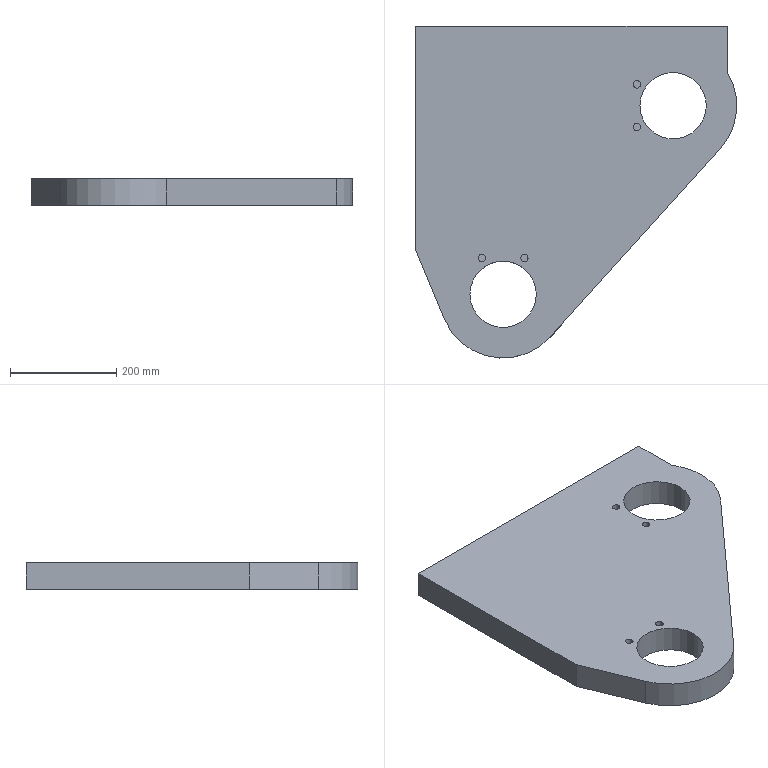Part | SolidWorks | features Cut 1, SplitBody 1 | 1 solid | 25 faces | box 605 x 625 x 50 mm | volume 12901911 mm3 | cylinder 14 | plane 11 | commonest cylinder face diameters 14 x8 125 x4 240 x2
STEP:
#1=CARTESIAN_POINT('',(3069.,481.749,-775.));
#2=VERTEX_POINT('',#1);
#3=CARTESIAN_POINT('',(3083.,481.749,-775.));
#4=VERTEX_POINT('',#3);
#5=CARTESIAN_POINT('',(3076.,481.749,-775.));
#6=DIRECTION('',(0.,0.,1.));
#7=DIRECTION('',(-1.,0.,0.));
#8=AXIS2_PLACEMENT_3D('',#5,#6,#7);
#9=CIRCLE('',#8,7.);
#10=EDGE_CURVE('',#2,#4,#9,.T.);
#11=ORIENTED_EDGE('',*,*,#10,.F.);
#12=CARTESIAN_POINT('',(3069.,481.749,-755.));
#13=VERTEX_POINT('',#12);
#14=CARTESIAN_POINT('',(3069.,481.749,-775.));
#15=DIRECTION('',(0.,0.,1.));
#16=VECTOR('',#15,1000.);
#17=LINE('',#14,#16);
#18=EDGE_CURVE('',#2,#13,#17,.T.);
#19=ORIENTED_EDGE('',*,*,#18,.T.);
#20=CARTESIAN_POINT('',(3083.,481.749,-755.));
#21=VERTEX_POINT('',#20);
#22=CARTESIAN_POINT('',(3076.,481.749,-755.));
#23=DIRECTION('',(0.,0.,1.));
#24=DIRECTION('',(-1.,0.,0.));
#25=AXIS2_PLACEMENT_3D('',#22,#23,#24);
#26=CIRCLE('',#25,7.);
#27=EDGE_CURVE('',#13,#21,#26,.T.);
#28=ORIENTED_EDGE('',*,*,#27,.T.);
#29=CARTESIAN_POINT('',(3083.,481.749,-775.));
#30=DIRECTION('',(0.,0.,1.));
#31=VECTOR('',#30,1000.);
#32=LINE('',#29,#31);
#33=EDGE_CURVE('',#4,#21,#32,.T.);
#34=ORIENTED_EDGE('',*,*,#33,.F.);
#35=EDGE_LOOP('',(#11,#19,#28,#34));
#36=FACE_OUTER_BOUND('',#35,.T.);
#37=CARTESIAN_POINT('',(3076.,481.749,-775.));
#38=DIRECTION('',(0.,0.,1.));
#39=DIRECTION('',(1.,0.,0.));
#40=AXIS2_PLACEMENT_3D('',#37,#38,#39);
#41=CYLINDRICAL_SURFACE('',#40,7.);
#42=ADVANCED_FACE('',(#36),#41,.F.);
#43=CARTESIAN_POINT('',(3149.,481.749,-775.));
#44=VERTEX_POINT('',#43);
#45=CARTESIAN_POINT('',(3163.,481.749,-775.));
#46=VERTEX_POINT('',#45);
#47=CARTESIAN_POINT('',(3156.,481.749,-775.));
#48=DIRECTION('',(0.,0.,1.));
#49=DIRECTION('',(1.,0.,0.));
#50=AXIS2_PLACEMENT_3D('',#47,#48,#49);
#51=CIRCLE('',#50,7.);
#52=EDGE_CURVE('',#44,#46,#51,.T.);
#53=ORIENTED_EDGE('',*,*,#52,.F.);
#54=CARTESIAN_POINT('',(3149.,481.749,-755.));
#55=VERTEX_POINT('',#54);
#56=CARTESIAN_POINT('',(3149.,481.749,-775.));
#57=DIRECTION('',(0.,0.,1.));
#58=VECTOR('',#57,1000.);
#59=LINE('',#56,#58);
#60=EDGE_CURVE('',#44,#55,#59,.T.);
#61=ORIENTED_EDGE('',*,*,#60,.T.);
#62=CARTESIAN_POINT('',(3163.,481.749,-755.));
#63=VERTEX_POINT('',#62);
#64=CARTESIAN_POINT('',(3156.,481.749,-755.));
#65=DIRECTION('',(0.,0.,1.));
#66=DIRECTION('',(1.,0.,0.));
#67=AXIS2_PLACEMENT_3D('',#64,#65,#66);
#68=CIRCLE('',#67,7.);
#69=EDGE_CURVE('',#55,#63,#68,.T.);
#70=ORIENTED_EDGE('',*,*,#69,.T.);
#71=CARTESIAN_POINT('',(3163.,481.749,-775.));
#72=DIRECTION('',(0.,0.,1.));
#73=VECTOR('',#72,1000.);
#74=LINE('',#71,#73);
#75=EDGE_CURVE('',#46,#63,#74,.T.);
#76=ORIENTED_EDGE('',*,*,#75,.F.);
#77=EDGE_LOOP('',(#53,#61,#70,#76));
#78=FACE_OUTER_BOUND('',#77,.T.);
#79=CARTESIAN_POINT('',(3156.,481.749,-775.));
#80=DIRECTION('',(0.,0.,1.));
#81=DIRECTION('',(1.,0.,0.));
#82=AXIS2_PLACEMENT_3D('',#79,#80,#81);
#83=CYLINDRICAL_SURFACE('',#82,7.);
#84=ADVANCED_FACE('',(#78),#83,.F.);
#85=CARTESIAN_POINT('',(3360.692,808.44,-775.));
#86=VERTEX_POINT('',#85);
#87=CARTESIAN_POINT('',(3374.692,808.44,-775.));
#88=VERTEX_POINT('',#87);
#89=CARTESIAN_POINT('',(3367.692,808.44,-775.));
#90=DIRECTION('',(0.,0.,1.));
#91=DIRECTION('',(1.,0.,0.));
#92=AXIS2_PLACEMENT_3D('',#89,#90,#91);
#93=CIRCLE('',#92,7.);
#94=EDGE_CURVE('',#86,#88,#93,.T.);
#95=ORIENTED_EDGE('',*,*,#94,.F.);
#96=CARTESIAN_POINT('',(3360.692,808.44,-755.));
#97=VERTEX_POINT('',#96);
#98=CARTESIAN_POINT('',(3360.692,808.44,-775.));
#99=DIRECTION('',(0.,0.,1.));
#100=VECTOR('',#99,1000.);
#101=LINE('',#98,#100);
#102=EDGE_CURVE('',#86,#97,#101,.T.);
#103=ORIENTED_EDGE('',*,*,#102,.T.);
#104=CARTESIAN_POINT('',(3374.692,808.44,-755.));
#105=VERTEX_POINT('',#104);
#106=CARTESIAN_POINT('',(3367.692,808.44,-755.));
#107=DIRECTION('',(0.,0.,1.));
#108=DIRECTION('',(1.,0.,0.));
#109=AXIS2_PLACEMENT_3D('',#106,#107,#108);
#110=CIRCLE('',#109,7.);
#111=EDGE_CURVE('',#97,#105,#110,.T.);
#112=ORIENTED_EDGE('',*,*,#111,.T.);
#113=CARTESIAN_POINT('',(3374.692,808.44,-775.));
#114=DIRECTION('',(0.,0.,1.));
#115=VECTOR('',#114,1000.);
#116=LINE('',#113,#115);
#117=EDGE_CURVE('',#88,#105,#116,.T.);
#118=ORIENTED_EDGE('',*,*,#117,.F.);
#119=EDGE_LOOP('',(#95,#103,#112,#118));
#120=FACE_OUTER_BOUND('',#119,.T.);
#121=CARTESIAN_POINT('',(3367.692,808.44,-775.));
#122=DIRECTION('',(0.,0.,1.));
#123=DIRECTION('',(1.,0.,0.));
#124=AXIS2_PLACEMENT_3D('',#121,#122,#123);
#125=CYLINDRICAL_SURFACE('',#124,7.);
#126=ADVANCED_FACE('',(#120),#125,.F.);
#127=CARTESIAN_POINT('',(3360.692,728.44,-775.));
#128=VERTEX_POINT('',#127);
#129=CARTESIAN_POINT('',(3374.692,728.44,-775.));
#130=VERTEX_POINT('',#129);
#131=CARTESIAN_POINT('',(3367.692,728.44,-775.));
#132=DIRECTION('',(0.,0.,1.));
#133=DIRECTION('',(1.,0.,0.));
#134=AXIS2_PLACEMENT_3D('',#131,#132,#133);
#135=CIRCLE('',#134,7.);
#136=EDGE_CURVE('',#128,#130,#135,.T.);
#137=ORIENTED_EDGE('',*,*,#136,.F.);
#138=CARTESIAN_POINT('',(3360.692,728.44,-755.));
#139=VERTEX_POINT('',#138);
#140=CARTESIAN_POINT('',(3360.692,728.44,-775.));
#141=DIRECTION('',(0.,0.,1.));
#142=VECTOR('',#141,1000.);
#143=LINE('',#140,#142);
#144=EDGE_CURVE('',#128,#139,#143,.T.);
#145=ORIENTED_EDGE('',*,*,#144,.T.);
#146=CARTESIAN_POINT('',(3374.692,728.44,-755.));
#147=VERTEX_POINT('',#146);
#148=CARTESIAN_POINT('',(3367.692,728.44,-755.));
#149=DIRECTION('',(0.,0.,1.));
#150=DIRECTION('',(1.,0.,0.));
#151=AXIS2_PLACEMENT_3D('',#148,#149,#150);
#152=CIRCLE('',#151,7.);
#153=EDGE_CURVE('',#139,#147,#152,.T.);
#154=ORIENTED_EDGE('',*,*,#153,.T.);
#155=CARTESIAN_POINT('',(3374.692,728.44,-775.));
#156=DIRECTION('',(0.,0.,1.));
#157=VECTOR('',#156,1000.);
#158=LINE('',#155,#157);
#159=EDGE_CURVE('',#130,#147,#158,.T.);
#160=ORIENTED_EDGE('',*,*,#159,.F.);
#161=EDGE_LOOP('',(#137,#145,#154,#160));
#162=FACE_OUTER_BOUND('',#161,.T.);
#163=CARTESIAN_POINT('',(3367.692,728.44,-775.));
#164=DIRECTION('',(0.,0.,1.));
#165=DIRECTION('',(1.,0.,0.));
#166=AXIS2_PLACEMENT_3D('',#163,#164,#165);
#167=CYLINDRICAL_SURFACE('',#166,7.);
#168=ADVANCED_FACE('',(#162),#167,.F.);
#169=CARTESIAN_POINT('',(3178.5,413.44,-755.));
#170=VERTEX_POINT('',#169);
#171=CARTESIAN_POINT('',(3053.5,413.44,-755.));
#172=VERTEX_POINT('',#171);
#173=CARTESIAN_POINT('',(3116.,413.44,-755.));
#174=DIRECTION('',(0.,0.,-1.));
#175=DIRECTION('',(-1.,0.,0.));
#176=AXIS2_PLACEMENT_3D('',#173,#174,#175);
#177=CIRCLE('',#176,62.5);
#178=EDGE_CURVE('',#170,#172,#177,.T.);
#179=ORIENTED_EDGE('',*,*,#178,.F.);
#180=CARTESIAN_POINT('',(3178.5,413.44,-805.));
#181=VERTEX_POINT('',#180);
#182=CARTESIAN_POINT('',(3178.5,413.44,-755.));
#183=DIRECTION('',(0.,0.,-1.));
#184=VECTOR('',#183,1000.);
#185=LINE('',#182,#184);
#186=EDGE_CURVE('',#170,#181,#185,.T.);
#187=ORIENTED_EDGE('',*,*,#186,.T.);
#188=CARTESIAN_POINT('',(3053.5,413.44,-805.));
#189=VERTEX_POINT('',#188);
#190=CARTESIAN_POINT('',(3116.,413.44,-805.));
#191=DIRECTION('',(0.,0.,1.));
#192=DIRECTION('',(-1.,0.,0.));
#193=AXIS2_PLACEMENT_3D('',#190,#191,#192);
#194=CIRCLE('',#193,62.5);
#195=EDGE_CURVE('',#189,#181,#194,.T.);
#196=ORIENTED_EDGE('',*,*,#195,.F.);
#197=CARTESIAN_POINT('',(3053.5,413.44,-755.));
#198=DIRECTION('',(0.,0.,-1.));
#199=VECTOR('',#198,1000.);
#200=LINE('',#197,#199);
#201=EDGE_CURVE('',#172,#189,#200,.T.);
#202=ORIENTED_EDGE('',*,*,#201,.F.);
#203=EDGE_LOOP('',(#179,#187,#196,#202));
#204=FACE_OUTER_BOUND('',#203,.T.);
#205=CARTESIAN_POINT('',(3116.,413.44,-755.));
#206=DIRECTION('',(0.,0.,-1.));
#207=DIRECTION('',(-1.,0.,0.));
#208=AXIS2_PLACEMENT_3D('',#205,#206,#207);
#209=CYLINDRICAL_SURFACE('',#208,62.5);
#210=ADVANCED_FACE('',(#204),#209,.F.);
#211=CARTESIAN_POINT('',(3498.5,768.44,-755.));
#212=VERTEX_POINT('',#211);
#213=CARTESIAN_POINT('',(3373.5,768.44,-755.));
#214=VERTEX_POINT('',#213);
#215=CARTESIAN_POINT('',(3436.,768.44,-755.));
#216=DIRECTION('',(0.,0.,-1.));
#217=DIRECTION('',(-1.,0.,0.));
#218=AXIS2_PLACEMENT_3D('',#215,#216,#217);
#219=CIRCLE('',#218,62.5);
#220=EDGE_CURVE('',#212,#214,#219,.T.);
#221=ORIENTED_EDGE('',*,*,#220,.F.);
#222=CARTESIAN_POINT('',(3498.5,768.44,-805.));
#223=VERTEX_POINT('',#222);
#224=CARTESIAN_POINT('',(3498.5,768.44,-755.));
#225=DIRECTION('',(0.,0.,-1.));
#226=VECTOR('',#225,1000.);
#227=LINE('',#224,#226);
#228=EDGE_CURVE('',#212,#223,#227,.T.);
#229=ORIENTED_EDGE('',*,*,#228,.T.);
#230=CARTESIAN_POINT('',(3373.5,768.44,-805.));
#231=VERTEX_POINT('',#230);
#232=CARTESIAN_POINT('',(3436.,768.44,-805.));
#233=DIRECTION('',(0.,0.,1.));
#234=DIRECTION('',(-1.,0.,0.));
#235=AXIS2_PLACEMENT_3D('',#232,#233,#234);
#236=CIRCLE('',#235,62.5);
#237=EDGE_CURVE('',#231,#223,#236,.T.);
#238=ORIENTED_EDGE('',*,*,#237,.F.);
#239=CARTESIAN_POINT('',(3373.5,768.44,-755.));
#240=DIRECTION('',(0.,0.,-1.));
#241=VECTOR('',#240,1000.);
#242=LINE('',#239,#241);
#243=EDGE_CURVE('',#214,#231,#242,.T.);
#244=ORIENTED_EDGE('',*,*,#243,.F.);
#245=EDGE_LOOP('',(#221,#229,#238,#244));
#246=FACE_OUTER_BOUND('',#245,.T.);
#247=CARTESIAN_POINT('',(3436.,768.44,-755.));
#248=DIRECTION('',(0.,0.,-1.));
#249=DIRECTION('',(-1.,0.,0.));
#250=AXIS2_PLACEMENT_3D('',#247,#248,#249);
#251=CYLINDRICAL_SURFACE('',#250,62.5);
#252=ADVANCED_FACE('',(#246),#251,.F.);
#253=CARTESIAN_POINT('',(3076.,481.749,-755.));
#254=DIRECTION('',(0.,0.,1.));
#255=DIRECTION('',(-1.,0.,0.));
#256=AXIS2_PLACEMENT_3D('',#253,#254,#255);
#257=CIRCLE('',#256,7.);
#258=EDGE_CURVE('',#21,#13,#257,.T.);
#259=ORIENTED_EDGE('',*,*,#258,.F.);
#260=ORIENTED_EDGE('',*,*,#27,.F.);
#261=EDGE_LOOP('',(#259,#260));
#262=FACE_BOUND('',#261,.T.);
#263=CARTESIAN_POINT('',(3156.,481.749,-755.));
#264=DIRECTION('',(0.,0.,1.));
#265=DIRECTION('',(1.,0.,0.));
#266=AXIS2_PLACEMENT_3D('',#263,#264,#265);
#267=CIRCLE('',#266,7.);
#268=EDGE_CURVE('',#63,#55,#267,.T.);
#269=ORIENTED_EDGE('',*,*,#268,.F.);
#270=ORIENTED_EDGE('',*,*,#69,.F.);
#271=EDGE_LOOP('',(#269,#270));
#272=FACE_BOUND('',#271,.T.);
#273=CARTESIAN_POINT('',(3367.692,808.44,-755.));
#274=DIRECTION('',(0.,0.,1.));
#275=DIRECTION('',(1.,0.,0.));
#276=AXIS2_PLACEMENT_3D('',#273,#274,#275);
#277=CIRCLE('',#276,7.);
#278=EDGE_CURVE('',#105,#97,#277,.T.);
#279=ORIENTED_EDGE('',*,*,#278,.F.);
#280=ORIENTED_EDGE('',*,*,#111,.F.);
#281=EDGE_LOOP('',(#279,#280));
#282=FACE_BOUND('',#281,.T.);
#283=CARTESIAN_POINT('',(3367.692,728.44,-755.));
#284=DIRECTION('',(0.,0.,1.));
#285=DIRECTION('',(1.,0.,0.));
#286=AXIS2_PLACEMENT_3D('',#283,#284,#285);
#287=CIRCLE('',#286,7.);
#288=EDGE_CURVE('',#147,#139,#287,.T.);
#289=ORIENTED_EDGE('',*,*,#288,.F.);
#290=ORIENTED_EDGE('',*,*,#153,.F.);
#291=EDGE_LOOP('',(#289,#290));
#292=FACE_BOUND('',#291,.T.);
#293=CARTESIAN_POINT('',(3116.,413.44,-755.));
#294=DIRECTION('',(0.,0.,-1.));
#295=DIRECTION('',(-1.,0.,0.));
#296=AXIS2_PLACEMENT_3D('',#293,#294,#295);
#297=CIRCLE('',#296,62.5);
#298=EDGE_CURVE('',#172,#170,#297,.T.);
#299=ORIENTED_EDGE('',*,*,#298,.T.);
#300=ORIENTED_EDGE('',*,*,#178,.T.);
#301=EDGE_LOOP('',(#299,#300));
#302=FACE_BOUND('',#301,.T.);
#303=CARTESIAN_POINT('',(2951.,918.44,-755.));
#304=VERTEX_POINT('',#303);
#305=CARTESIAN_POINT('',(2951.,498.44,-755.));
#306=VERTEX_POINT('',#305);
#307=CARTESIAN_POINT('',(2951.,413.44,-755.));
#308=DIRECTION('',(0.,-1.,0.));
#309=VECTOR('',#308,1000.);
#310=LINE('',#307,#309);
#311=EDGE_CURVE('',#304,#306,#310,.T.);
#312=ORIENTED_EDGE('',*,*,#311,.T.);
#313=CARTESIAN_POINT('',(3005.106,367.587,-755.));
#314=VERTEX_POINT('',#313);
#315=CARTESIAN_POINT('',(2951.,498.44,-755.));
#316=DIRECTION('',(0.3821,-0.9241,0.));
#317=VECTOR('',#316,1000.);
#318=LINE('',#315,#317);
#319=EDGE_CURVE('',#306,#314,#318,.T.);
#320=ORIENTED_EDGE('',*,*,#319,.T.);
#321=CARTESIAN_POINT('',(3205.133,333.095,-755.));
#322=VERTEX_POINT('',#321);
#323=CARTESIAN_POINT('',(3116.,413.44,-755.));
#324=DIRECTION('',(0.,0.,1.));
#325=DIRECTION('',(-1.,0.,0.));
#326=AXIS2_PLACEMENT_3D('',#323,#324,#325);
#327=CIRCLE('',#326,120.);
#328=EDGE_CURVE('',#314,#322,#327,.T.);
#329=ORIENTED_EDGE('',*,*,#328,.T.);
#330=CARTESIAN_POINT('',(3525.133,688.095,-755.));
#331=VERTEX_POINT('',#330);
#332=CARTESIAN_POINT('',(3205.133,333.095,-755.));
#333=DIRECTION('',(0.6695,0.7428,0.));
#334=VECTOR('',#333,1000.);
#335=LINE('',#332,#334);
#336=EDGE_CURVE('',#322,#331,#335,.T.);
#337=ORIENTED_EDGE('',*,*,#336,.T.);
#338=CARTESIAN_POINT('',(3538.,831.654,-755.));
#339=VERTEX_POINT('',#338);
#340=CARTESIAN_POINT('',(3436.,768.44,-755.));
#341=DIRECTION('',(0.,0.,1.));
#342=DIRECTION('',(-1.,0.,0.));
#343=AXIS2_PLACEMENT_3D('',#340,#341,#342);
#344=CIRCLE('',#343,120.);
#345=EDGE_CURVE('',#331,#339,#344,.T.);
#346=ORIENTED_EDGE('',*,*,#345,.T.);
#347=CARTESIAN_POINT('',(3538.,918.44,-755.));
#348=VERTEX_POINT('',#347);
#349=CARTESIAN_POINT('',(3538.,413.44,-755.));
#350=DIRECTION('',(0.,1.,0.));
#351=VECTOR('',#350,1000.);
#352=LINE('',#349,#351);
#353=EDGE_CURVE('',#339,#348,#352,.T.);
#354=ORIENTED_EDGE('',*,*,#353,.T.);
#355=CARTESIAN_POINT('',(3116.,918.44,-755.));
#356=DIRECTION('',(-1.,0.,0.));
#357=VECTOR('',#356,1000.);
#358=LINE('',#355,#357);
#359=EDGE_CURVE('',#348,#304,#358,.T.);
#360=ORIENTED_EDGE('',*,*,#359,.T.);
#361=EDGE_LOOP('',(#312,#320,#329,#337,#346,#354,#360));
#362=FACE_OUTER_BOUND('',#361,.T.);
#363=CARTESIAN_POINT('',(3436.,768.44,-755.));
#364=DIRECTION('',(0.,0.,-1.));
#365=DIRECTION('',(-1.,0.,0.));
#366=AXIS2_PLACEMENT_3D('',#363,#364,#365);
#367=CIRCLE('',#366,62.5);
#368=EDGE_CURVE('',#214,#212,#367,.T.);
#369=ORIENTED_EDGE('',*,*,#368,.T.);
#370=ORIENTED_EDGE('',*,*,#220,.T.);
#371=EDGE_LOOP('',(#369,#370));
#372=FACE_BOUND('',#371,.T.);
#373=CARTESIAN_POINT('',(3116.,413.44,-755.));
#374=DIRECTION('',(0.,0.,1.));
#375=DIRECTION('',(1.,0.,0.));
#376=AXIS2_PLACEMENT_3D('',#373,#374,#375);
#377=PLANE('',#376);
#378=ADVANCED_FACE('',(#262,#272,#282,#292,#302,#362,#372),#377,.T.);
#379=ORIENTED_EDGE('',*,*,#186,.F.);
#380=ORIENTED_EDGE('',*,*,#298,.F.);
#381=ORIENTED_EDGE('',*,*,#201,.T.);
#382=CARTESIAN_POINT('',(3116.,413.44,-805.));
#383=DIRECTION('',(0.,0.,1.));
#384=DIRECTION('',(-1.,0.,0.));
#385=AXIS2_PLACEMENT_3D('',#382,#383,#384);
#386=CIRCLE('',#385,62.5);
#387=EDGE_CURVE('',#181,#189,#386,.T.);
#388=ORIENTED_EDGE('',*,*,#387,.F.);
#389=EDGE_LOOP('',(#379,#380,#381,#388));
#390=FACE_OUTER_BOUND('',#389,.T.);
#391=CARTESIAN_POINT('',(3116.,413.44,-755.));
#392=DIRECTION('',(0.,0.,-1.));
#393=DIRECTION('',(-1.,0.,0.));
#394=AXIS2_PLACEMENT_3D('',#391,#392,#393);
#395=CYLINDRICAL_SURFACE('',#394,62.5);
#396=ADVANCED_FACE('',(#390),#395,.F.);
#397=CARTESIAN_POINT('',(3005.106,367.587,-805.));
#398=VERTEX_POINT('',#397);
#399=CARTESIAN_POINT('',(3005.106,367.587,-755.));
#400=DIRECTION('',(0.,0.,-1.));
#401=VECTOR('',#400,1000.);
#402=LINE('',#399,#401);
#403=EDGE_CURVE('',#314,#398,#402,.T.);
#404=ORIENTED_EDGE('',*,*,#403,.F.);
#405=ORIENTED_EDGE('',*,*,#319,.F.);
#406=CARTESIAN_POINT('',(2951.,498.44,-805.));
#407=VERTEX_POINT('',#406);
#408=CARTESIAN_POINT('',(2951.,498.44,-755.));
#409=DIRECTION('',(0.,0.,1.));
#410=VECTOR('',#409,1000.);
#411=LINE('',#408,#410);
#412=EDGE_CURVE('',#407,#306,#411,.T.);
#413=ORIENTED_EDGE('',*,*,#412,.F.);
#414=CARTESIAN_POINT('',(2951.,498.44,-805.));
#415=DIRECTION('',(-0.3821,0.9241,0.));
#416=VECTOR('',#415,1000.);
#417=LINE('',#414,#416);
#418=EDGE_CURVE('',#398,#407,#417,.T.);
#419=ORIENTED_EDGE('',*,*,#418,.F.);
#420=EDGE_LOOP('',(#404,#405,#413,#419));
#421=FACE_OUTER_BOUND('',#420,.T.);
#422=CARTESIAN_POINT('',(2951.,498.44,-755.));
#423=DIRECTION('',(0.9241,0.3821,0.));
#424=DIRECTION('',(-0.3821,0.9241,0.));
#425=AXIS2_PLACEMENT_3D('',#422,#423,#424);
#426=PLANE('',#425);
#427=ADVANCED_FACE('',(#421),#426,.F.);
#428=ORIENTED_EDGE('',*,*,#412,.T.);
#429=ORIENTED_EDGE('',*,*,#311,.F.);
#430=CARTESIAN_POINT('',(2951.,918.44,-805.));
#431=VERTEX_POINT('',#430);
#432=CARTESIAN_POINT('',(2951.,918.44,-755.));
#433=DIRECTION('',(0.,0.,1.));
#434=VECTOR('',#433,1000.);
#435=LINE('',#432,#434);
#436=EDGE_CURVE('',#431,#304,#435,.T.);
#437=ORIENTED_EDGE('',*,*,#436,.F.);
#438=CARTESIAN_POINT('',(2951.,498.44,-805.));
#439=DIRECTION('',(0.,1.,0.));
#440=VECTOR('',#439,1000.);
#441=LINE('',#438,#440);
#442=EDGE_CURVE('',#407,#431,#441,.T.);
#443=ORIENTED_EDGE('',*,*,#442,.F.);
#444=EDGE_LOOP('',(#428,#429,#437,#443));
#445=FACE_OUTER_BOUND('',#444,.T.);
#446=CARTESIAN_POINT('',(2951.,498.44,-755.));
#447=DIRECTION('',(1.,0.,0.));
#448=DIRECTION('',(0.,0.,-1.));
#449=AXIS2_PLACEMENT_3D('',#446,#447,#448);
#450=PLANE('',#449);
#451=ADVANCED_FACE('',(#445),#450,.F.);
#452=ORIENTED_EDGE('',*,*,#436,.T.);
#453=ORIENTED_EDGE('',*,*,#359,.F.);
#454=CARTESIAN_POINT('',(3538.,918.44,-805.));
#455=VERTEX_POINT('',#454);
#456=CARTESIAN_POINT('',(3538.,918.44,-755.));
#457=DIRECTION('',(0.,0.,1.));
#458=VECTOR('',#457,1000.);
#459=LINE('',#456,#458);
#460=EDGE_CURVE('',#455,#348,#459,.T.);
#461=ORIENTED_EDGE('',*,*,#460,.F.);
#462=CARTESIAN_POINT('',(2951.,918.44,-805.));
#463=DIRECTION('',(1.,0.,0.));
#464=VECTOR('',#463,1000.);
#465=LINE('',#462,#464);
#466=EDGE_CURVE('',#431,#455,#465,.T.);
#467=ORIENTED_EDGE('',*,*,#466,.F.);
#468=EDGE_LOOP('',(#452,#453,#461,#467));
#469=FACE_OUTER_BOUND('',#468,.T.);
#470=CARTESIAN_POINT('',(2951.,918.44,-755.));
#471=DIRECTION('',(0.,-1.,0.));
#472=DIRECTION('',(1.,0.,0.));
#473=AXIS2_PLACEMENT_3D('',#470,#471,#472);
#474=PLANE('',#473);
#475=ADVANCED_FACE('',(#469),#474,.F.);
#476=ORIENTED_EDGE('',*,*,#460,.T.);
#477=ORIENTED_EDGE('',*,*,#353,.F.);
#478=CARTESIAN_POINT('',(3538.,831.654,-805.));
#479=VERTEX_POINT('',#478);
#480=CARTESIAN_POINT('',(3538.,831.654,-755.));
#481=DIRECTION('',(0.,0.,1.));
#482=VECTOR('',#481,1000.);
#483=LINE('',#480,#482);
#484=EDGE_CURVE('',#479,#339,#483,.T.);
#485=ORIENTED_EDGE('',*,*,#484,.F.);
#486=CARTESIAN_POINT('',(3538.,918.44,-805.));
#487=DIRECTION('',(0.,-1.,0.));
#488=VECTOR('',#487,1000.);
#489=LINE('',#486,#488);
#490=EDGE_CURVE('',#455,#479,#489,.T.);
#491=ORIENTED_EDGE('',*,*,#490,.F.);
#492=EDGE_LOOP('',(#476,#477,#485,#491));
#493=FACE_OUTER_BOUND('',#492,.T.);
#494=CARTESIAN_POINT('',(3538.,918.44,-755.));
#495=DIRECTION('',(-1.,0.,0.));
#496=DIRECTION('',(0.,-1.,0.));
#497=AXIS2_PLACEMENT_3D('',#494,#495,#496);
#498=PLANE('',#497);
#499=ADVANCED_FACE('',(#493),#498,.F.);
#500=ORIENTED_EDGE('',*,*,#345,.F.);
#501=CARTESIAN_POINT('',(3525.133,688.095,-805.));
#502=VERTEX_POINT('',#501);
#503=CARTESIAN_POINT('',(3525.133,688.095,-755.));
#504=DIRECTION('',(0.,0.,-1.));
#505=VECTOR('',#504,1000.);
#506=LINE('',#503,#505);
#507=EDGE_CURVE('',#331,#502,#506,.T.);
#508=ORIENTED_EDGE('',*,*,#507,.T.);
#509=CARTESIAN_POINT('',(3436.,768.44,-805.));
#510=DIRECTION('',(0.,0.,1.));
#511=DIRECTION('',(-1.,0.,0.));
#512=AXIS2_PLACEMENT_3D('',#509,#510,#511);
#513=CIRCLE('',#512,120.);
#514=EDGE_CURVE('',#502,#479,#513,.T.);
#515=ORIENTED_EDGE('',*,*,#514,.T.);
#516=ORIENTED_EDGE('',*,*,#484,.T.);
#517=EDGE_LOOP('',(#500,#508,#515,#516));
#518=FACE_OUTER_BOUND('',#517,.T.);
#519=CARTESIAN_POINT('',(3436.,768.44,-755.));
#520=DIRECTION('',(0.,0.,-1.));
#521=DIRECTION('',(-1.,0.,0.));
#522=AXIS2_PLACEMENT_3D('',#519,#520,#521);
#523=CYLINDRICAL_SURFACE('',#522,120.);
#524=ADVANCED_FACE('',(#518),#523,.T.);
#525=ORIENTED_EDGE('',*,*,#507,.F.);
#526=ORIENTED_EDGE('',*,*,#336,.F.);
#527=CARTESIAN_POINT('',(3205.133,333.095,-805.));
#528=VERTEX_POINT('',#527);
#529=CARTESIAN_POINT('',(3205.133,333.095,-755.));
#530=DIRECTION('',(0.,0.,1.));
#531=VECTOR('',#530,1000.);
#532=LINE('',#529,#531);
#533=EDGE_CURVE('',#528,#322,#532,.T.);
#534=ORIENTED_EDGE('',*,*,#533,.F.);
#535=CARTESIAN_POINT('',(3205.133,333.095,-805.));
#536=DIRECTION('',(-0.6695,-0.7428,0.));
#537=VECTOR('',#536,1000.);
#538=LINE('',#535,#537);
#539=EDGE_CURVE('',#502,#528,#538,.T.);
#540=ORIENTED_EDGE('',*,*,#539,.F.);
#541=EDGE_LOOP('',(#525,#526,#534,#540));
#542=FACE_OUTER_BOUND('',#541,.T.);
#543=CARTESIAN_POINT('',(3205.133,333.095,-755.));
#544=DIRECTION('',(-0.7428,0.6695,0.));
#545=DIRECTION('',(-0.6695,-0.7428,0.));
#546=AXIS2_PLACEMENT_3D('',#543,#544,#545);
#547=PLANE('',#546);
#548=ADVANCED_FACE('',(#542),#547,.F.);
#549=ORIENTED_EDGE('',*,*,#328,.F.);
#550=ORIENTED_EDGE('',*,*,#403,.T.);
#551=CARTESIAN_POINT('',(3116.,413.44,-805.));
#552=DIRECTION('',(0.,0.,1.));
#553=DIRECTION('',(-1.,0.,0.));
#554=AXIS2_PLACEMENT_3D('',#551,#552,#553);
#555=CIRCLE('',#554,120.);
#556=EDGE_CURVE('',#398,#528,#555,.T.);
#557=ORIENTED_EDGE('',*,*,#556,.T.);
#558=ORIENTED_EDGE('',*,*,#533,.T.);
#559=EDGE_LOOP('',(#549,#550,#557,#558));
#560=FACE_OUTER_BOUND('',#559,.T.);
#561=CARTESIAN_POINT('',(3116.,413.44,-755.));
#562=DIRECTION('',(0.,0.,-1.));
#563=DIRECTION('',(-1.,0.,0.));
#564=AXIS2_PLACEMENT_3D('',#561,#562,#563);
#565=CYLINDRICAL_SURFACE('',#564,120.);
#566=ADVANCED_FACE('',(#560),#565,.T.);
#567=ORIENTED_EDGE('',*,*,#228,.F.);
#568=ORIENTED_EDGE('',*,*,#368,.F.);
#569=ORIENTED_EDGE('',*,*,#243,.T.);
#570=CARTESIAN_POINT('',(3436.,768.44,-805.));
#571=DIRECTION('',(0.,0.,1.));
#572=DIRECTION('',(-1.,0.,0.));
#573=AXIS2_PLACEMENT_3D('',#570,#571,#572);
#574=CIRCLE('',#573,62.5);
#575=EDGE_CURVE('',#223,#231,#574,.T.);
#576=ORIENTED_EDGE('',*,*,#575,.F.);
#577=EDGE_LOOP('',(#567,#568,#569,#576));
#578=FACE_OUTER_BOUND('',#577,.T.);
#579=CARTESIAN_POINT('',(3436.,768.44,-755.));
#580=DIRECTION('',(0.,0.,-1.));
#581=DIRECTION('',(-1.,0.,0.));
#582=AXIS2_PLACEMENT_3D('',#579,#580,#581);
#583=CYLINDRICAL_SURFACE('',#582,62.5);
#584=ADVANCED_FACE('',(#578),#583,.F.);
#585=ORIENTED_EDGE('',*,*,#195,.T.);
#586=ORIENTED_EDGE('',*,*,#387,.T.);
#587=EDGE_LOOP('',(#585,#586));
#588=FACE_BOUND('',#587,.T.);
#589=ORIENTED_EDGE('',*,*,#418,.T.);
#590=ORIENTED_EDGE('',*,*,#442,.T.);
#591=ORIENTED_EDGE('',*,*,#466,.T.);
#592=ORIENTED_EDGE('',*,*,#490,.T.);
#593=ORIENTED_EDGE('',*,*,#514,.F.);
#594=ORIENTED_EDGE('',*,*,#539,.T.);
#595=ORIENTED_EDGE('',*,*,#556,.F.);
#596=EDGE_LOOP('',(#589,#590,#591,#592,#593,#594,#595));
#597=FACE_OUTER_BOUND('',#596,.T.);
#598=ORIENTED_EDGE('',*,*,#237,.T.);
#599=ORIENTED_EDGE('',*,*,#575,.T.);
#600=EDGE_LOOP('',(#598,#599));
#601=FACE_BOUND('',#600,.T.);
#602=CARTESIAN_POINT('',(3116.,413.44,-805.));
#603=DIRECTION('',(0.,0.,1.));
#604=DIRECTION('',(1.,0.,0.));
#605=AXIS2_PLACEMENT_3D('',#602,#603,#604);
#606=PLANE('',#605);
#607=ADVANCED_FACE('',(#588,#597,#601),#606,.F.);
#608=ORIENTED_EDGE('',*,*,#144,.F.);
#609=CARTESIAN_POINT('',(3367.692,728.44,-775.));
#610=DIRECTION('',(0.,0.,1.));
#611=DIRECTION('',(1.,0.,0.));
#612=AXIS2_PLACEMENT_3D('',#609,#610,#611);
#613=CIRCLE('',#612,7.);
#614=EDGE_CURVE('',#130,#128,#613,.T.);
#615=ORIENTED_EDGE('',*,*,#614,.F.);
#616=ORIENTED_EDGE('',*,*,#159,.T.);
#617=ORIENTED_EDGE('',*,*,#288,.T.);
#618=EDGE_LOOP('',(#608,#615,#616,#617));
#619=FACE_OUTER_BOUND('',#618,.T.);
#620=CARTESIAN_POINT('',(3367.692,728.44,-775.));
#621=DIRECTION('',(0.,0.,1.));
#622=DIRECTION('',(1.,0.,0.));
#623=AXIS2_PLACEMENT_3D('',#620,#621,#622);
#624=CYLINDRICAL_SURFACE('',#623,7.);
#625=ADVANCED_FACE('',(#619),#624,.F.);
#626=ORIENTED_EDGE('',*,*,#614,.T.);
#627=ORIENTED_EDGE('',*,*,#136,.T.);
#628=EDGE_LOOP('',(#626,#627));
#629=FACE_OUTER_BOUND('',#628,.T.);
#630=CARTESIAN_POINT('',(3367.692,728.44,-775.));
#631=DIRECTION('',(0.,0.,1.));
#632=DIRECTION('',(1.,0.,0.));
#633=AXIS2_PLACEMENT_3D('',#630,#631,#632);
#634=PLANE('',#633);
#635=ADVANCED_FACE('',(#629),#634,.T.);
#636=ORIENTED_EDGE('',*,*,#102,.F.);
#637=CARTESIAN_POINT('',(3367.692,808.44,-775.));
#638=DIRECTION('',(0.,0.,1.));
#639=DIRECTION('',(1.,0.,0.));
#640=AXIS2_PLACEMENT_3D('',#637,#638,#639);
#641=CIRCLE('',#640,7.);
#642=EDGE_CURVE('',#88,#86,#641,.T.);
#643=ORIENTED_EDGE('',*,*,#642,.F.);
#644=ORIENTED_EDGE('',*,*,#117,.T.);
#645=ORIENTED_EDGE('',*,*,#278,.T.);
#646=EDGE_LOOP('',(#636,#643,#644,#645));
#647=FACE_OUTER_BOUND('',#646,.T.);
#648=CARTESIAN_POINT('',(3367.692,808.44,-775.));
#649=DIRECTION('',(0.,0.,1.));
#650=DIRECTION('',(1.,0.,0.));
#651=AXIS2_PLACEMENT_3D('',#648,#649,#650);
#652=CYLINDRICAL_SURFACE('',#651,7.);
#653=ADVANCED_FACE('',(#647),#652,.F.);
#654=ORIENTED_EDGE('',*,*,#642,.T.);
#655=ORIENTED_EDGE('',*,*,#94,.T.);
#656=EDGE_LOOP('',(#654,#655));
#657=FACE_OUTER_BOUND('',#656,.T.);
#658=CARTESIAN_POINT('',(3367.692,808.44,-775.));
#659=DIRECTION('',(0.,0.,1.));
#660=DIRECTION('',(1.,0.,0.));
#661=AXIS2_PLACEMENT_3D('',#658,#659,#660);
#662=PLANE('',#661);
#663=ADVANCED_FACE('',(#657),#662,.T.);
#664=ORIENTED_EDGE('',*,*,#60,.F.);
#665=CARTESIAN_POINT('',(3156.,481.749,-775.));
#666=DIRECTION('',(0.,0.,1.));
#667=DIRECTION('',(1.,0.,0.));
#668=AXIS2_PLACEMENT_3D('',#665,#666,#667);
#669=CIRCLE('',#668,7.);
#670=EDGE_CURVE('',#46,#44,#669,.T.);
#671=ORIENTED_EDGE('',*,*,#670,.F.);
#672=ORIENTED_EDGE('',*,*,#75,.T.);
#673=ORIENTED_EDGE('',*,*,#268,.T.);
#674=EDGE_LOOP('',(#664,#671,#672,#673));
#675=FACE_OUTER_BOUND('',#674,.T.);
#676=CARTESIAN_POINT('',(3156.,481.749,-775.));
#677=DIRECTION('',(0.,0.,1.));
#678=DIRECTION('',(1.,0.,0.));
#679=AXIS2_PLACEMENT_3D('',#676,#677,#678);
#680=CYLINDRICAL_SURFACE('',#679,7.);
#681=ADVANCED_FACE('',(#675),#680,.F.);
#682=ORIENTED_EDGE('',*,*,#670,.T.);
#683=ORIENTED_EDGE('',*,*,#52,.T.);
#684=EDGE_LOOP('',(#682,#683));
#685=FACE_OUTER_BOUND('',#684,.T.);
#686=CARTESIAN_POINT('',(3156.,481.749,-775.));
#687=DIRECTION('',(0.,0.,1.));
#688=DIRECTION('',(1.,0.,0.));
#689=AXIS2_PLACEMENT_3D('',#686,#687,#688);
#690=PLANE('',#689);
#691=ADVANCED_FACE('',(#685),#690,.T.);
#692=ORIENTED_EDGE('',*,*,#18,.F.);
#693=CARTESIAN_POINT('',(3076.,481.749,-775.));
#694=DIRECTION('',(0.,0.,1.));
#695=DIRECTION('',(-1.,0.,0.));
#696=AXIS2_PLACEMENT_3D('',#693,#694,#695);
#697=CIRCLE('',#696,7.);
#698=EDGE_CURVE('',#4,#2,#697,.T.);
#699=ORIENTED_EDGE('',*,*,#698,.F.);
#700=ORIENTED_EDGE('',*,*,#33,.T.);
#701=ORIENTED_EDGE('',*,*,#258,.T.);
#702=EDGE_LOOP('',(#692,#699,#700,#701));
#703=FACE_OUTER_BOUND('',#702,.T.);
#704=CARTESIAN_POINT('',(3076.,481.749,-775.));
#705=DIRECTION('',(0.,0.,1.));
#706=DIRECTION('',(1.,0.,0.));
#707=AXIS2_PLACEMENT_3D('',#704,#705,#706);
#708=CYLINDRICAL_SURFACE('',#707,7.);
#709=ADVANCED_FACE('',(#703),#708,.F.);
#710=ORIENTED_EDGE('',*,*,#698,.T.);
#711=ORIENTED_EDGE('',*,*,#10,.T.);
#712=EDGE_LOOP('',(#710,#711));
#713=FACE_OUTER_BOUND('',#712,.T.);
#714=CARTESIAN_POINT('',(3076.,481.749,-775.));
#715=DIRECTION('',(0.,0.,-1.));
#716=DIRECTION('',(-1.,0.,0.));
#717=AXIS2_PLACEMENT_3D('',#714,#715,#716);
#718=PLANE('',#717);
#719=ADVANCED_FACE('',(#713),#718,.F.);
#720=CLOSED_SHELL('',(#42,#84,#126,#168,#210,#252,#378,#396,#427,#451,#475,#499,#524,#548,#566,#584,#607,#625,#635,#653,#663,#681,#691,#709,#719));
#721=MANIFOLD_SOLID_BREP('',#720);
#722=CARTESIAN_POINT('',(0.,0.,0.));
#723=DIRECTION('',(0.,0.,1.));
#724=DIRECTION('',(1.,0.,0.));
#725=AXIS2_PLACEMENT_3D('',#722,#723,#724);
#726=(LENGTH_UNIT()NAMED_UNIT(*)SI_UNIT(.MILLI.,.METRE.));
#727=UNCERTAINTY_MEASURE_WITH_UNIT(LENGTH_MEASURE(0.00001),#726,'','');
#728=(NAMED_UNIT(*)PLANE_ANGLE_UNIT()SI_UNIT($,.RADIAN.));
#729=(NAMED_UNIT(*)SI_UNIT($,.STERADIAN.)SOLID_ANGLE_UNIT());
#730=(GEOMETRIC_REPRESENTATION_CONTEXT(3)GLOBAL_UNCERTAINTY_ASSIGNED_CONTEXT((#727))GLOBAL_UNIT_ASSIGNED_CONTEXT((#726,#728,#729))REPRESENTATION_CONTEXT('',''));
#731=ADVANCED_BREP_SHAPE_REPRESENTATION('',(#721,#725),#730);